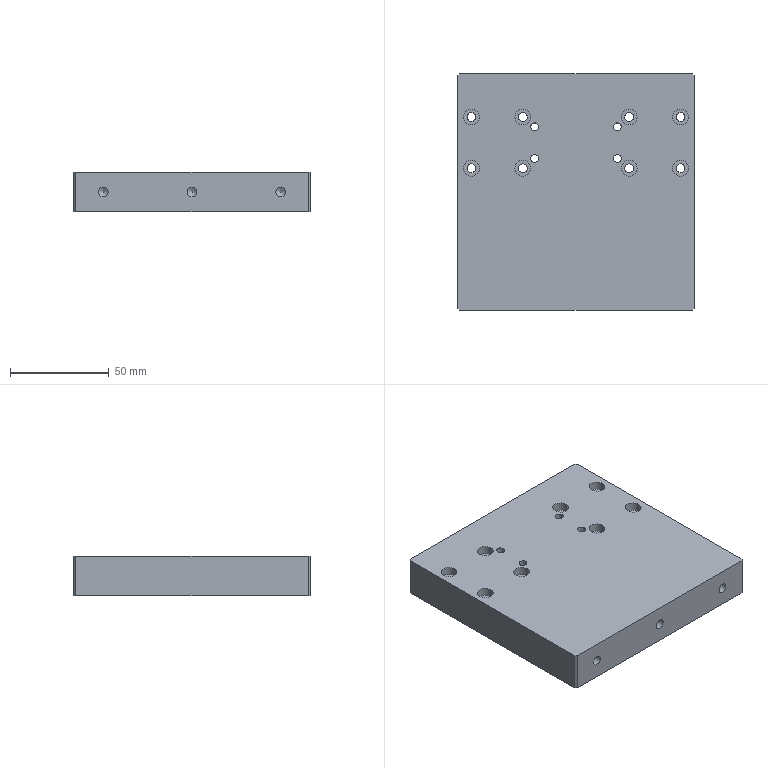Part | 1 solid | 52 faces | box 120 x 120 x 20 mm | volume 280448 mm3 | cylinder 27 | plane 18 | cone 7 | commonest cylinder face diameters 4.5 x8 8 x8 4 x4 5 x3 4.2 x2 6.8 x2
STEP:
#1=CARTESIAN_POINT('',(-59.,60.,10.));
#2=VERTEX_POINT('',#1);
#3=CARTESIAN_POINT('',(-60.,59.,10.));
#4=VERTEX_POINT('',#3);
#5=CARTESIAN_POINT('',(-59.5,59.5,10.));
#6=DIRECTION('',(-0.7071,-0.7071,0.));
#7=VECTOR('',#6,1000.);
#8=LINE('',#5,#7);
#9=EDGE_CURVE('',#2,#4,#8,.T.);
#10=ORIENTED_EDGE('',*,*,#9,.F.);
#11=CARTESIAN_POINT('',(-59.,60.,-10.));
#12=VERTEX_POINT('',#11);
#13=CARTESIAN_POINT('',(-59.,60.,10.));
#14=DIRECTION('',(0.,0.,1.));
#15=VECTOR('',#14,1000.);
#16=LINE('',#13,#15);
#17=EDGE_CURVE('',#12,#2,#16,.T.);
#18=ORIENTED_EDGE('',*,*,#17,.F.);
#19=CARTESIAN_POINT('',(-60.,59.,-10.));
#20=VERTEX_POINT('',#19);
#21=CARTESIAN_POINT('',(-60.,59.,-10.));
#22=DIRECTION('',(0.7071,0.7071,0.));
#23=VECTOR('',#22,1000.);
#24=LINE('',#21,#23);
#25=EDGE_CURVE('',#20,#12,#24,.T.);
#26=ORIENTED_EDGE('',*,*,#25,.F.);
#27=CARTESIAN_POINT('',(-60.,59.,10.));
#28=DIRECTION('',(0.,0.,-1.));
#29=VECTOR('',#28,1000.);
#30=LINE('',#27,#29);
#31=EDGE_CURVE('',#4,#20,#30,.T.);
#32=ORIENTED_EDGE('',*,*,#31,.F.);
#33=EDGE_LOOP('',(#10,#18,#26,#32));
#34=FACE_BOUND('',#33,.T.);
#35=CARTESIAN_POINT('',(-60.,59.,10.));
#36=DIRECTION('',(0.7071,-0.7071,0.));
#37=DIRECTION('',(0.,0.,-1.));
#38=AXIS2_PLACEMENT_3D('',#35,#36,#37);
#39=PLANE('',#38);
#40=ADVANCED_FACE('',(#34),#39,.F.);
#41=CARTESIAN_POINT('',(-60.,-59.,10.));
#42=VERTEX_POINT('',#41);
#43=CARTESIAN_POINT('',(-59.,-60.,10.));
#44=VERTEX_POINT('',#43);
#45=CARTESIAN_POINT('',(-59.5,-59.5,10.));
#46=DIRECTION('',(0.7071,-0.7071,0.));
#47=VECTOR('',#46,1000.);
#48=LINE('',#45,#47);
#49=EDGE_CURVE('',#42,#44,#48,.T.);
#50=ORIENTED_EDGE('',*,*,#49,.F.);
#51=CARTESIAN_POINT('',(-60.,-59.,-10.));
#52=VERTEX_POINT('',#51);
#53=CARTESIAN_POINT('',(-60.,-59.,10.));
#54=DIRECTION('',(0.,0.,1.));
#55=VECTOR('',#54,1000.);
#56=LINE('',#53,#55);
#57=EDGE_CURVE('',#52,#42,#56,.T.);
#58=ORIENTED_EDGE('',*,*,#57,.F.);
#59=CARTESIAN_POINT('',(-59.,-60.,-10.));
#60=VERTEX_POINT('',#59);
#61=CARTESIAN_POINT('',(-59.,-60.,-10.));
#62=DIRECTION('',(-0.7071,0.7071,0.));
#63=VECTOR('',#62,1000.);
#64=LINE('',#61,#63);
#65=EDGE_CURVE('',#60,#52,#64,.T.);
#66=ORIENTED_EDGE('',*,*,#65,.F.);
#67=CARTESIAN_POINT('',(-59.,-60.,10.));
#68=DIRECTION('',(0.,0.,-1.));
#69=VECTOR('',#68,1000.);
#70=LINE('',#67,#69);
#71=EDGE_CURVE('',#44,#60,#70,.T.);
#72=ORIENTED_EDGE('',*,*,#71,.F.);
#73=EDGE_LOOP('',(#50,#58,#66,#72));
#74=FACE_BOUND('',#73,.T.);
#75=CARTESIAN_POINT('',(-59.,-60.,10.));
#76=DIRECTION('',(0.7071,0.7071,0.));
#77=DIRECTION('',(0.,0.,-1.));
#78=AXIS2_PLACEMENT_3D('',#75,#76,#77);
#79=PLANE('',#78);
#80=ADVANCED_FACE('',(#74),#79,.F.);
#81=CARTESIAN_POINT('',(59.,-60.,10.));
#82=VERTEX_POINT('',#81);
#83=CARTESIAN_POINT('',(60.,-59.,10.));
#84=VERTEX_POINT('',#83);
#85=CARTESIAN_POINT('',(59.5,-59.5,10.));
#86=DIRECTION('',(0.7071,0.7071,0.));
#87=VECTOR('',#86,1000.);
#88=LINE('',#85,#87);
#89=EDGE_CURVE('',#82,#84,#88,.T.);
#90=ORIENTED_EDGE('',*,*,#89,.F.);
#91=CARTESIAN_POINT('',(59.,-60.,-10.));
#92=VERTEX_POINT('',#91);
#93=CARTESIAN_POINT('',(59.,-60.,10.));
#94=DIRECTION('',(0.,0.,1.));
#95=VECTOR('',#94,1000.);
#96=LINE('',#93,#95);
#97=EDGE_CURVE('',#92,#82,#96,.T.);
#98=ORIENTED_EDGE('',*,*,#97,.F.);
#99=CARTESIAN_POINT('',(60.,-59.,-10.));
#100=VERTEX_POINT('',#99);
#101=CARTESIAN_POINT('',(60.,-59.,-10.));
#102=DIRECTION('',(-0.7071,-0.7071,0.));
#103=VECTOR('',#102,1000.);
#104=LINE('',#101,#103);
#105=EDGE_CURVE('',#100,#92,#104,.T.);
#106=ORIENTED_EDGE('',*,*,#105,.F.);
#107=CARTESIAN_POINT('',(60.,-59.,10.));
#108=DIRECTION('',(0.,0.,-1.));
#109=VECTOR('',#108,1000.);
#110=LINE('',#107,#109);
#111=EDGE_CURVE('',#84,#100,#110,.T.);
#112=ORIENTED_EDGE('',*,*,#111,.F.);
#113=EDGE_LOOP('',(#90,#98,#106,#112));
#114=FACE_BOUND('',#113,.T.);
#115=CARTESIAN_POINT('',(60.,-59.,10.));
#116=DIRECTION('',(-0.7071,0.7071,0.));
#117=DIRECTION('',(0.,0.,-1.));
#118=AXIS2_PLACEMENT_3D('',#115,#116,#117);
#119=PLANE('',#118);
#120=ADVANCED_FACE('',(#114),#119,.F.);
#121=CARTESIAN_POINT('',(60.,59.,10.));
#122=VERTEX_POINT('',#121);
#123=CARTESIAN_POINT('',(59.,60.,10.));
#124=VERTEX_POINT('',#123);
#125=CARTESIAN_POINT('',(59.5,59.5,10.));
#126=DIRECTION('',(-0.7071,0.7071,0.));
#127=VECTOR('',#126,1000.);
#128=LINE('',#125,#127);
#129=EDGE_CURVE('',#122,#124,#128,.T.);
#130=ORIENTED_EDGE('',*,*,#129,.F.);
#131=CARTESIAN_POINT('',(60.,59.,-10.));
#132=VERTEX_POINT('',#131);
#133=CARTESIAN_POINT('',(60.,59.,10.));
#134=DIRECTION('',(0.,0.,1.));
#135=VECTOR('',#134,1000.);
#136=LINE('',#133,#135);
#137=EDGE_CURVE('',#132,#122,#136,.T.);
#138=ORIENTED_EDGE('',*,*,#137,.F.);
#139=CARTESIAN_POINT('',(59.,60.,-10.));
#140=VERTEX_POINT('',#139);
#141=CARTESIAN_POINT('',(59.,60.,-10.));
#142=DIRECTION('',(0.7071,-0.7071,0.));
#143=VECTOR('',#142,1000.);
#144=LINE('',#141,#143);
#145=EDGE_CURVE('',#140,#132,#144,.T.);
#146=ORIENTED_EDGE('',*,*,#145,.F.);
#147=CARTESIAN_POINT('',(59.,60.,10.));
#148=DIRECTION('',(0.,0.,-1.));
#149=VECTOR('',#148,1000.);
#150=LINE('',#147,#149);
#151=EDGE_CURVE('',#124,#140,#150,.T.);
#152=ORIENTED_EDGE('',*,*,#151,.F.);
#153=EDGE_LOOP('',(#130,#138,#146,#152));
#154=FACE_BOUND('',#153,.T.);
#155=CARTESIAN_POINT('',(59.,60.,10.));
#156=DIRECTION('',(-0.7071,-0.7071,0.));
#157=DIRECTION('',(0.,0.,-1.));
#158=AXIS2_PLACEMENT_3D('',#155,#156,#157);
#159=PLANE('',#158);
#160=ADVANCED_FACE('',(#154),#159,.F.);
#161=CARTESIAN_POINT('',(-49.,38.,5.6));
#162=VERTEX_POINT('',#161);
#163=CARTESIAN_POINT('',(-53.,38.,5.6));
#164=DIRECTION('',(0.,0.,1.));
#165=DIRECTION('',(1.,0.,0.));
#166=AXIS2_PLACEMENT_3D('',#163,#164,#165);
#167=CIRCLE('',#166,4.);
#168=EDGE_CURVE('',#162,#162,#167,.T.);
#169=ORIENTED_EDGE('',*,*,#168,.T.);
#170=EDGE_LOOP('',(#169));
#171=FACE_BOUND('',#170,.T.);
#172=CARTESIAN_POINT('',(-50.75,38.,5.6));
#173=VERTEX_POINT('',#172);
#174=CARTESIAN_POINT('',(-53.,38.,5.6));
#175=DIRECTION('',(0.,0.,1.));
#176=DIRECTION('',(1.,0.,0.));
#177=AXIS2_PLACEMENT_3D('',#174,#175,#176);
#178=CIRCLE('',#177,2.25);
#179=EDGE_CURVE('',#173,#173,#178,.T.);
#180=ORIENTED_EDGE('',*,*,#179,.F.);
#181=EDGE_LOOP('',(#180));
#182=FACE_BOUND('',#181,.T.);
#183=CARTESIAN_POINT('',(-50.75,38.,5.6));
#184=DIRECTION('',(0.,0.,-1.));
#185=DIRECTION('',(-1.,0.,0.));
#186=AXIS2_PLACEMENT_3D('',#183,#184,#185);
#187=PLANE('',#186);
#188=ADVANCED_FACE('',(#171,#182),#187,.F.);
#189=CARTESIAN_POINT('',(-57.,12.,5.6));
#190=VERTEX_POINT('',#189);
#191=CARTESIAN_POINT('',(-53.,12.,5.6));
#192=DIRECTION('',(0.,0.,1.));
#193=DIRECTION('',(-1.,0.,0.));
#194=AXIS2_PLACEMENT_3D('',#191,#192,#193);
#195=CIRCLE('',#194,4.);
#196=EDGE_CURVE('',#190,#190,#195,.T.);
#197=ORIENTED_EDGE('',*,*,#196,.T.);
#198=EDGE_LOOP('',(#197));
#199=FACE_BOUND('',#198,.T.);
#200=CARTESIAN_POINT('',(-55.25,12.,5.6));
#201=VERTEX_POINT('',#200);
#202=CARTESIAN_POINT('',(-53.,12.,5.6));
#203=DIRECTION('',(0.,0.,1.));
#204=DIRECTION('',(-1.,0.,0.));
#205=AXIS2_PLACEMENT_3D('',#202,#203,#204);
#206=CIRCLE('',#205,2.25);
#207=EDGE_CURVE('',#201,#201,#206,.T.);
#208=ORIENTED_EDGE('',*,*,#207,.F.);
#209=EDGE_LOOP('',(#208));
#210=FACE_BOUND('',#209,.T.);
#211=CARTESIAN_POINT('',(-50.75,38.,5.6));
#212=DIRECTION('',(0.,0.,-1.));
#213=DIRECTION('',(-1.,0.,0.));
#214=AXIS2_PLACEMENT_3D('',#211,#212,#213);
#215=PLANE('',#214);
#216=ADVANCED_FACE('',(#199,#210),#215,.F.);
#217=CARTESIAN_POINT('',(-31.,12.,5.6));
#218=VERTEX_POINT('',#217);
#219=CARTESIAN_POINT('',(-27.,12.,5.6));
#220=DIRECTION('',(0.,0.,1.));
#221=DIRECTION('',(-1.,0.,0.));
#222=AXIS2_PLACEMENT_3D('',#219,#220,#221);
#223=CIRCLE('',#222,4.);
#224=EDGE_CURVE('',#218,#218,#223,.T.);
#225=ORIENTED_EDGE('',*,*,#224,.T.);
#226=EDGE_LOOP('',(#225));
#227=FACE_BOUND('',#226,.T.);
#228=CARTESIAN_POINT('',(-29.25,12.,5.6));
#229=VERTEX_POINT('',#228);
#230=CARTESIAN_POINT('',(-27.,12.,5.6));
#231=DIRECTION('',(0.,0.,1.));
#232=DIRECTION('',(-1.,0.,0.));
#233=AXIS2_PLACEMENT_3D('',#230,#231,#232);
#234=CIRCLE('',#233,2.25);
#235=EDGE_CURVE('',#229,#229,#234,.T.);
#236=ORIENTED_EDGE('',*,*,#235,.F.);
#237=EDGE_LOOP('',(#236));
#238=FACE_BOUND('',#237,.T.);
#239=CARTESIAN_POINT('',(-50.75,38.,5.6));
#240=DIRECTION('',(0.,0.,-1.));
#241=DIRECTION('',(-1.,0.,0.));
#242=AXIS2_PLACEMENT_3D('',#239,#240,#241);
#243=PLANE('',#242);
#244=ADVANCED_FACE('',(#227,#238),#243,.F.);
#245=CARTESIAN_POINT('',(-31.,38.,5.6));
#246=VERTEX_POINT('',#245);
#247=CARTESIAN_POINT('',(-27.,38.,5.6));
#248=DIRECTION('',(0.,0.,1.));
#249=DIRECTION('',(-1.,0.,0.));
#250=AXIS2_PLACEMENT_3D('',#247,#248,#249);
#251=CIRCLE('',#250,4.);
#252=EDGE_CURVE('',#246,#246,#251,.T.);
#253=ORIENTED_EDGE('',*,*,#252,.T.);
#254=EDGE_LOOP('',(#253));
#255=FACE_BOUND('',#254,.T.);
#256=CARTESIAN_POINT('',(-29.25,38.,5.6));
#257=VERTEX_POINT('',#256);
#258=CARTESIAN_POINT('',(-27.,38.,5.6));
#259=DIRECTION('',(0.,0.,1.));
#260=DIRECTION('',(-1.,0.,0.));
#261=AXIS2_PLACEMENT_3D('',#258,#259,#260);
#262=CIRCLE('',#261,2.25);
#263=EDGE_CURVE('',#257,#257,#262,.T.);
#264=ORIENTED_EDGE('',*,*,#263,.F.);
#265=EDGE_LOOP('',(#264));
#266=FACE_BOUND('',#265,.T.);
#267=CARTESIAN_POINT('',(-50.75,38.,5.6));
#268=DIRECTION('',(0.,0.,-1.));
#269=DIRECTION('',(-1.,0.,0.));
#270=AXIS2_PLACEMENT_3D('',#267,#268,#269);
#271=PLANE('',#270);
#272=ADVANCED_FACE('',(#255,#266),#271,.F.);
#273=CARTESIAN_POINT('',(23.,38.,5.6));
#274=VERTEX_POINT('',#273);
#275=CARTESIAN_POINT('',(27.,38.,5.6));
#276=DIRECTION('',(0.,0.,1.));
#277=DIRECTION('',(-1.,0.,0.));
#278=AXIS2_PLACEMENT_3D('',#275,#276,#277);
#279=CIRCLE('',#278,4.);
#280=EDGE_CURVE('',#274,#274,#279,.T.);
#281=ORIENTED_EDGE('',*,*,#280,.T.);
#282=EDGE_LOOP('',(#281));
#283=FACE_BOUND('',#282,.T.);
#284=CARTESIAN_POINT('',(24.75,38.,5.6));
#285=VERTEX_POINT('',#284);
#286=CARTESIAN_POINT('',(27.,38.,5.6));
#287=DIRECTION('',(0.,0.,1.));
#288=DIRECTION('',(-1.,0.,0.));
#289=AXIS2_PLACEMENT_3D('',#286,#287,#288);
#290=CIRCLE('',#289,2.25);
#291=EDGE_CURVE('',#285,#285,#290,.T.);
#292=ORIENTED_EDGE('',*,*,#291,.F.);
#293=EDGE_LOOP('',(#292));
#294=FACE_BOUND('',#293,.T.);
#295=CARTESIAN_POINT('',(-50.75,38.,5.6));
#296=DIRECTION('',(0.,0.,-1.));
#297=DIRECTION('',(-1.,0.,0.));
#298=AXIS2_PLACEMENT_3D('',#295,#296,#297);
#299=PLANE('',#298);
#300=ADVANCED_FACE('',(#283,#294),#299,.F.);
#301=CARTESIAN_POINT('',(23.,12.,5.6));
#302=VERTEX_POINT('',#301);
#303=CARTESIAN_POINT('',(27.,12.,5.6));
#304=DIRECTION('',(0.,0.,1.));
#305=DIRECTION('',(-1.,0.,0.));
#306=AXIS2_PLACEMENT_3D('',#303,#304,#305);
#307=CIRCLE('',#306,4.);
#308=EDGE_CURVE('',#302,#302,#307,.T.);
#309=ORIENTED_EDGE('',*,*,#308,.T.);
#310=EDGE_LOOP('',(#309));
#311=FACE_BOUND('',#310,.T.);
#312=CARTESIAN_POINT('',(24.75,12.,5.6));
#313=VERTEX_POINT('',#312);
#314=CARTESIAN_POINT('',(27.,12.,5.6));
#315=DIRECTION('',(0.,0.,1.));
#316=DIRECTION('',(-1.,0.,0.));
#317=AXIS2_PLACEMENT_3D('',#314,#315,#316);
#318=CIRCLE('',#317,2.25);
#319=EDGE_CURVE('',#313,#313,#318,.T.);
#320=ORIENTED_EDGE('',*,*,#319,.F.);
#321=EDGE_LOOP('',(#320));
#322=FACE_BOUND('',#321,.T.);
#323=CARTESIAN_POINT('',(-50.75,38.,5.6));
#324=DIRECTION('',(0.,0.,-1.));
#325=DIRECTION('',(-1.,0.,0.));
#326=AXIS2_PLACEMENT_3D('',#323,#324,#325);
#327=PLANE('',#326);
#328=ADVANCED_FACE('',(#311,#322),#327,.F.);
#329=CARTESIAN_POINT('',(49.,12.,5.6));
#330=VERTEX_POINT('',#329);
#331=CARTESIAN_POINT('',(53.,12.,5.6));
#332=DIRECTION('',(0.,0.,1.));
#333=DIRECTION('',(-1.,0.,0.));
#334=AXIS2_PLACEMENT_3D('',#331,#332,#333);
#335=CIRCLE('',#334,4.);
#336=EDGE_CURVE('',#330,#330,#335,.T.);
#337=ORIENTED_EDGE('',*,*,#336,.T.);
#338=EDGE_LOOP('',(#337));
#339=FACE_BOUND('',#338,.T.);
#340=CARTESIAN_POINT('',(50.75,12.,5.6));
#341=VERTEX_POINT('',#340);
#342=CARTESIAN_POINT('',(53.,12.,5.6));
#343=DIRECTION('',(0.,0.,1.));
#344=DIRECTION('',(-1.,0.,0.));
#345=AXIS2_PLACEMENT_3D('',#342,#343,#344);
#346=CIRCLE('',#345,2.25);
#347=EDGE_CURVE('',#341,#341,#346,.T.);
#348=ORIENTED_EDGE('',*,*,#347,.F.);
#349=EDGE_LOOP('',(#348));
#350=FACE_BOUND('',#349,.T.);
#351=CARTESIAN_POINT('',(-50.75,38.,5.6));
#352=DIRECTION('',(0.,0.,-1.));
#353=DIRECTION('',(-1.,0.,0.));
#354=AXIS2_PLACEMENT_3D('',#351,#352,#353);
#355=PLANE('',#354);
#356=ADVANCED_FACE('',(#339,#350),#355,.F.);
#357=CARTESIAN_POINT('',(49.,38.,5.6));
#358=VERTEX_POINT('',#357);
#359=CARTESIAN_POINT('',(53.,38.,5.6));
#360=DIRECTION('',(0.,0.,1.));
#361=DIRECTION('',(-1.,0.,0.));
#362=AXIS2_PLACEMENT_3D('',#359,#360,#361);
#363=CIRCLE('',#362,4.);
#364=EDGE_CURVE('',#358,#358,#363,.T.);
#365=ORIENTED_EDGE('',*,*,#364,.T.);
#366=EDGE_LOOP('',(#365));
#367=FACE_BOUND('',#366,.T.);
#368=CARTESIAN_POINT('',(50.75,38.,5.6));
#369=VERTEX_POINT('',#368);
#370=CARTESIAN_POINT('',(53.,38.,5.6));
#371=DIRECTION('',(0.,0.,1.));
#372=DIRECTION('',(-1.,0.,0.));
#373=AXIS2_PLACEMENT_3D('',#370,#371,#372);
#374=CIRCLE('',#373,2.25);
#375=EDGE_CURVE('',#369,#369,#374,.T.);
#376=ORIENTED_EDGE('',*,*,#375,.F.);
#377=EDGE_LOOP('',(#376));
#378=FACE_BOUND('',#377,.T.);
#379=CARTESIAN_POINT('',(-50.75,38.,5.6));
#380=DIRECTION('',(0.,0.,-1.));
#381=DIRECTION('',(-1.,0.,0.));
#382=AXIS2_PLACEMENT_3D('',#379,#380,#381);
#383=PLANE('',#382);
#384=ADVANCED_FACE('',(#367,#378),#383,.F.);
#385=CARTESIAN_POINT('',(60.,60.,-10.));
#386=DIRECTION('',(-1.,0.,0.));
#387=VECTOR('',#386,1000.);
#388=LINE('',#385,#387);
#389=EDGE_CURVE('',#140,#12,#388,.T.);
#390=ORIENTED_EDGE('',*,*,#389,.F.);
#391=ORIENTED_EDGE('',*,*,#145,.T.);
#392=CARTESIAN_POINT('',(60.,-60.,-10.));
#393=DIRECTION('',(0.,1.,0.));
#394=VECTOR('',#393,1000.);
#395=LINE('',#392,#394);
#396=EDGE_CURVE('',#100,#132,#395,.T.);
#397=ORIENTED_EDGE('',*,*,#396,.F.);
#398=ORIENTED_EDGE('',*,*,#105,.T.);
#399=CARTESIAN_POINT('',(60.,-60.,-10.));
#400=DIRECTION('',(1.,0.,0.));
#401=VECTOR('',#400,1000.);
#402=LINE('',#399,#401);
#403=EDGE_CURVE('',#60,#92,#402,.T.);
#404=ORIENTED_EDGE('',*,*,#403,.F.);
#405=ORIENTED_EDGE('',*,*,#65,.T.);
#406=CARTESIAN_POINT('',(-60.,-60.,-10.));
#407=DIRECTION('',(0.,-1.,0.));
#408=VECTOR('',#407,1000.);
#409=LINE('',#406,#408);
#410=EDGE_CURVE('',#20,#52,#409,.T.);
#411=ORIENTED_EDGE('',*,*,#410,.F.);
#412=ORIENTED_EDGE('',*,*,#25,.T.);
#413=EDGE_LOOP('',(#390,#391,#397,#398,#404,#405,#411,#412));
#414=FACE_BOUND('',#413,.T.);
#415=CARTESIAN_POINT('',(55.25,38.,-10.));
#416=VERTEX_POINT('',#415);
#417=CARTESIAN_POINT('',(53.,38.,-10.));
#418=DIRECTION('',(0.,0.,1.));
#419=DIRECTION('',(1.,0.,0.));
#420=AXIS2_PLACEMENT_3D('',#417,#418,#419);
#421=CIRCLE('',#420,2.25);
#422=EDGE_CURVE('',#416,#416,#421,.T.);
#423=ORIENTED_EDGE('',*,*,#422,.T.);
#424=EDGE_LOOP('',(#423));
#425=FACE_BOUND('',#424,.T.);
#426=CARTESIAN_POINT('',(55.25,12.,-10.));
#427=VERTEX_POINT('',#426);
#428=CARTESIAN_POINT('',(53.,12.,-10.));
#429=DIRECTION('',(0.,0.,1.));
#430=DIRECTION('',(1.,0.,0.));
#431=AXIS2_PLACEMENT_3D('',#428,#429,#430);
#432=CIRCLE('',#431,2.25);
#433=EDGE_CURVE('',#427,#427,#432,.T.);
#434=ORIENTED_EDGE('',*,*,#433,.T.);
#435=EDGE_LOOP('',(#434));
#436=FACE_BOUND('',#435,.T.);
#437=CARTESIAN_POINT('',(29.25,12.,-10.));
#438=VERTEX_POINT('',#437);
#439=CARTESIAN_POINT('',(27.,12.,-10.));
#440=DIRECTION('',(0.,0.,1.));
#441=DIRECTION('',(1.,0.,0.));
#442=AXIS2_PLACEMENT_3D('',#439,#440,#441);
#443=CIRCLE('',#442,2.25);
#444=EDGE_CURVE('',#438,#438,#443,.T.);
#445=ORIENTED_EDGE('',*,*,#444,.T.);
#446=EDGE_LOOP('',(#445));
#447=FACE_BOUND('',#446,.T.);
#448=CARTESIAN_POINT('',(29.25,38.,-10.));
#449=VERTEX_POINT('',#448);
#450=CARTESIAN_POINT('',(27.,38.,-10.));
#451=DIRECTION('',(0.,0.,1.));
#452=DIRECTION('',(1.,0.,0.));
#453=AXIS2_PLACEMENT_3D('',#450,#451,#452);
#454=CIRCLE('',#453,2.25);
#455=EDGE_CURVE('',#449,#449,#454,.T.);
#456=ORIENTED_EDGE('',*,*,#455,.T.);
#457=EDGE_LOOP('',(#456));
#458=FACE_BOUND('',#457,.T.);
#459=CARTESIAN_POINT('',(-24.75,38.,-10.));
#460=VERTEX_POINT('',#459);
#461=CARTESIAN_POINT('',(-27.,38.,-10.));
#462=DIRECTION('',(0.,0.,1.));
#463=DIRECTION('',(1.,0.,0.));
#464=AXIS2_PLACEMENT_3D('',#461,#462,#463);
#465=CIRCLE('',#464,2.25);
#466=EDGE_CURVE('',#460,#460,#465,.T.);
#467=ORIENTED_EDGE('',*,*,#466,.T.);
#468=EDGE_LOOP('',(#467));
#469=FACE_BOUND('',#468,.T.);
#470=CARTESIAN_POINT('',(-24.75,12.,-10.));
#471=VERTEX_POINT('',#470);
#472=CARTESIAN_POINT('',(-27.,12.,-10.));
#473=DIRECTION('',(0.,0.,1.));
#474=DIRECTION('',(1.,0.,0.));
#475=AXIS2_PLACEMENT_3D('',#472,#473,#474);
#476=CIRCLE('',#475,2.25);
#477=EDGE_CURVE('',#471,#471,#476,.T.);
#478=ORIENTED_EDGE('',*,*,#477,.T.);
#479=EDGE_LOOP('',(#478));
#480=FACE_BOUND('',#479,.T.);
#481=CARTESIAN_POINT('',(-50.75,12.,-10.));
#482=VERTEX_POINT('',#481);
#483=CARTESIAN_POINT('',(-53.,12.,-10.));
#484=DIRECTION('',(0.,0.,1.));
#485=DIRECTION('',(1.,0.,0.));
#486=AXIS2_PLACEMENT_3D('',#483,#484,#485);
#487=CIRCLE('',#486,2.25);
#488=EDGE_CURVE('',#482,#482,#487,.T.);
#489=ORIENTED_EDGE('',*,*,#488,.T.);
#490=EDGE_LOOP('',(#489));
#491=FACE_BOUND('',#490,.T.);
#492=CARTESIAN_POINT('',(-50.75,38.,-10.));
#493=VERTEX_POINT('',#492);
#494=CARTESIAN_POINT('',(-53.,38.,-10.));
#495=DIRECTION('',(0.,0.,1.));
#496=DIRECTION('',(1.,0.,0.));
#497=AXIS2_PLACEMENT_3D('',#494,#495,#496);
#498=CIRCLE('',#497,2.25);
#499=EDGE_CURVE('',#493,#493,#498,.T.);
#500=ORIENTED_EDGE('',*,*,#499,.T.);
#501=EDGE_LOOP('',(#500));
#502=FACE_BOUND('',#501,.T.);
#503=CARTESIAN_POINT('',(23.,17.,-10.));
#504=VERTEX_POINT('',#503);
#505=CARTESIAN_POINT('',(21.,17.,-10.));
#506=DIRECTION('',(0.,0.,1.));
#507=DIRECTION('',(1.,0.,0.));
#508=AXIS2_PLACEMENT_3D('',#505,#506,#507);
#509=CIRCLE('',#508,2.);
#510=EDGE_CURVE('',#504,#504,#509,.T.);
#511=ORIENTED_EDGE('',*,*,#510,.T.);
#512=EDGE_LOOP('',(#511));
#513=FACE_BOUND('',#512,.T.);
#514=CARTESIAN_POINT('',(23.,33.,-10.));
#515=VERTEX_POINT('',#514);
#516=CARTESIAN_POINT('',(21.,33.,-10.));
#517=DIRECTION('',(0.,0.,1.));
#518=DIRECTION('',(1.,0.,0.));
#519=AXIS2_PLACEMENT_3D('',#516,#517,#518);
#520=CIRCLE('',#519,2.);
#521=EDGE_CURVE('',#515,#515,#520,.T.);
#522=ORIENTED_EDGE('',*,*,#521,.T.);
#523=EDGE_LOOP('',(#522));
#524=FACE_BOUND('',#523,.T.);
#525=CARTESIAN_POINT('',(-19.,17.,-10.));
#526=VERTEX_POINT('',#525);
#527=CARTESIAN_POINT('',(-21.,17.,-10.));
#528=DIRECTION('',(0.,0.,1.));
#529=DIRECTION('',(1.,0.,0.));
#530=AXIS2_PLACEMENT_3D('',#527,#528,#529);
#531=CIRCLE('',#530,2.);
#532=EDGE_CURVE('',#526,#526,#531,.T.);
#533=ORIENTED_EDGE('',*,*,#532,.T.);
#534=EDGE_LOOP('',(#533));
#535=FACE_BOUND('',#534,.T.);
#536=CARTESIAN_POINT('',(-19.,33.,-10.));
#537=VERTEX_POINT('',#536);
#538=CARTESIAN_POINT('',(-21.,33.,-10.));
#539=DIRECTION('',(0.,0.,1.));
#540=DIRECTION('',(1.,0.,0.));
#541=AXIS2_PLACEMENT_3D('',#538,#539,#540);
#542=CIRCLE('',#541,2.);
#543=EDGE_CURVE('',#537,#537,#542,.T.);
#544=ORIENTED_EDGE('',*,*,#543,.T.);
#545=EDGE_LOOP('',(#544));
#546=FACE_BOUND('',#545,.T.);
#547=CARTESIAN_POINT('',(0.,0.,-10.));
#548=DIRECTION('',(0.,0.,1.));
#549=DIRECTION('',(1.,0.,0.));
#550=AXIS2_PLACEMENT_3D('',#547,#548,#549);
#551=PLANE('',#550);
#552=ADVANCED_FACE('',(#414,#425,#436,#447,#458,#469,#480,#491,#502,#513,#524,#535,#546),#551,.F.);
#553=CARTESIAN_POINT('',(60.,-60.,10.));
#554=DIRECTION('',(0.,1.,0.));
#555=VECTOR('',#554,1000.);
#556=LINE('',#553,#555);
#557=EDGE_CURVE('',#84,#122,#556,.T.);
#558=ORIENTED_EDGE('',*,*,#557,.T.);
#559=ORIENTED_EDGE('',*,*,#129,.T.);
#560=CARTESIAN_POINT('',(60.,60.,10.));
#561=DIRECTION('',(-1.,0.,0.));
#562=VECTOR('',#561,1000.);
#563=LINE('',#560,#562);
#564=EDGE_CURVE('',#124,#2,#563,.T.);
#565=ORIENTED_EDGE('',*,*,#564,.T.);
#566=ORIENTED_EDGE('',*,*,#9,.T.);
#567=CARTESIAN_POINT('',(-60.,-60.,10.));
#568=DIRECTION('',(0.,-1.,0.));
#569=VECTOR('',#568,1000.);
#570=LINE('',#567,#569);
#571=EDGE_CURVE('',#4,#42,#570,.T.);
#572=ORIENTED_EDGE('',*,*,#571,.T.);
#573=ORIENTED_EDGE('',*,*,#49,.T.);
#574=CARTESIAN_POINT('',(60.,-60.,10.));
#575=DIRECTION('',(1.,0.,0.));
#576=VECTOR('',#575,1000.);
#577=LINE('',#574,#576);
#578=EDGE_CURVE('',#44,#82,#577,.T.);
#579=ORIENTED_EDGE('',*,*,#578,.T.);
#580=ORIENTED_EDGE('',*,*,#89,.T.);
#581=EDGE_LOOP('',(#558,#559,#565,#566,#572,#573,#579,#580));
#582=FACE_BOUND('',#581,.T.);
#583=CARTESIAN_POINT('',(57.,38.,10.));
#584=VERTEX_POINT('',#583);
#585=CARTESIAN_POINT('',(53.,38.,10.));
#586=DIRECTION('',(0.,0.,1.));
#587=DIRECTION('',(1.,0.,0.));
#588=AXIS2_PLACEMENT_3D('',#585,#586,#587);
#589=CIRCLE('',#588,4.);
#590=EDGE_CURVE('',#584,#584,#589,.T.);
#591=ORIENTED_EDGE('',*,*,#590,.F.);
#592=EDGE_LOOP('',(#591));
#593=FACE_BOUND('',#592,.T.);
#594=CARTESIAN_POINT('',(57.,12.,10.));
#595=VERTEX_POINT('',#594);
#596=CARTESIAN_POINT('',(53.,12.,10.));
#597=DIRECTION('',(0.,0.,1.));
#598=DIRECTION('',(1.,0.,0.));
#599=AXIS2_PLACEMENT_3D('',#596,#597,#598);
#600=CIRCLE('',#599,4.);
#601=EDGE_CURVE('',#595,#595,#600,.T.);
#602=ORIENTED_EDGE('',*,*,#601,.F.);
#603=EDGE_LOOP('',(#602));
#604=FACE_BOUND('',#603,.T.);
#605=CARTESIAN_POINT('',(31.,12.,10.));
#606=VERTEX_POINT('',#605);
#607=CARTESIAN_POINT('',(27.,12.,10.));
#608=DIRECTION('',(0.,0.,1.));
#609=DIRECTION('',(1.,0.,0.));
#610=AXIS2_PLACEMENT_3D('',#607,#608,#609);
#611=CIRCLE('',#610,4.);
#612=EDGE_CURVE('',#606,#606,#611,.T.);
#613=ORIENTED_EDGE('',*,*,#612,.F.);
#614=EDGE_LOOP('',(#613));
#615=FACE_BOUND('',#614,.T.);
#616=CARTESIAN_POINT('',(31.,38.,10.));
#617=VERTEX_POINT('',#616);
#618=CARTESIAN_POINT('',(27.,38.,10.));
#619=DIRECTION('',(0.,0.,1.));
#620=DIRECTION('',(1.,0.,0.));
#621=AXIS2_PLACEMENT_3D('',#618,#619,#620);
#622=CIRCLE('',#621,4.);
#623=EDGE_CURVE('',#617,#617,#622,.T.);
#624=ORIENTED_EDGE('',*,*,#623,.F.);
#625=EDGE_LOOP('',(#624));
#626=FACE_BOUND('',#625,.T.);
#627=CARTESIAN_POINT('',(-23.,38.,10.));
#628=VERTEX_POINT('',#627);
#629=CARTESIAN_POINT('',(-27.,38.,10.));
#630=DIRECTION('',(0.,0.,1.));
#631=DIRECTION('',(1.,0.,0.));
#632=AXIS2_PLACEMENT_3D('',#629,#630,#631);
#633=CIRCLE('',#632,4.);
#634=EDGE_CURVE('',#628,#628,#633,.T.);
#635=ORIENTED_EDGE('',*,*,#634,.F.);
#636=EDGE_LOOP('',(#635));
#637=FACE_BOUND('',#636,.T.);
#638=CARTESIAN_POINT('',(-23.,12.,10.));
#639=VERTEX_POINT('',#638);
#640=CARTESIAN_POINT('',(-27.,12.,10.));
#641=DIRECTION('',(0.,0.,1.));
#642=DIRECTION('',(1.,0.,0.));
#643=AXIS2_PLACEMENT_3D('',#640,#641,#642);
#644=CIRCLE('',#643,4.);
#645=EDGE_CURVE('',#639,#639,#644,.T.);
#646=ORIENTED_EDGE('',*,*,#645,.F.);
#647=EDGE_LOOP('',(#646));
#648=FACE_BOUND('',#647,.T.);
#649=CARTESIAN_POINT('',(-49.,12.,10.));
#650=VERTEX_POINT('',#649);
#651=CARTESIAN_POINT('',(-53.,12.,10.));
#652=DIRECTION('',(0.,0.,1.));
#653=DIRECTION('',(1.,0.,0.));
#654=AXIS2_PLACEMENT_3D('',#651,#652,#653);
#655=CIRCLE('',#654,4.);
#656=EDGE_CURVE('',#650,#650,#655,.T.);
#657=ORIENTED_EDGE('',*,*,#656,.F.);
#658=EDGE_LOOP('',(#657));
#659=FACE_BOUND('',#658,.T.);
#660=CARTESIAN_POINT('',(-49.,38.,10.));
#661=VERTEX_POINT('',#660);
#662=CARTESIAN_POINT('',(-53.,38.,10.));
#663=DIRECTION('',(0.,0.,1.));
#664=DIRECTION('',(1.,0.,0.));
#665=AXIS2_PLACEMENT_3D('',#662,#663,#664);
#666=CIRCLE('',#665,4.);
#667=EDGE_CURVE('',#661,#661,#666,.T.);
#668=ORIENTED_EDGE('',*,*,#667,.F.);
#669=EDGE_LOOP('',(#668));
#670=FACE_BOUND('',#669,.T.);
#671=CARTESIAN_POINT('',(23.,17.,10.));
#672=VERTEX_POINT('',#671);
#673=CARTESIAN_POINT('',(21.,17.,10.));
#674=DIRECTION('',(0.,0.,1.));
#675=DIRECTION('',(1.,0.,0.));
#676=AXIS2_PLACEMENT_3D('',#673,#674,#675);
#677=CIRCLE('',#676,2.);
#678=EDGE_CURVE('',#672,#672,#677,.T.);
#679=ORIENTED_EDGE('',*,*,#678,.F.);
#680=EDGE_LOOP('',(#679));
#681=FACE_BOUND('',#680,.T.);
#682=CARTESIAN_POINT('',(23.,33.,10.));
#683=VERTEX_POINT('',#682);
#684=CARTESIAN_POINT('',(21.,33.,10.));
#685=DIRECTION('',(0.,0.,1.));
#686=DIRECTION('',(1.,0.,0.));
#687=AXIS2_PLACEMENT_3D('',#684,#685,#686);
#688=CIRCLE('',#687,2.);
#689=EDGE_CURVE('',#683,#683,#688,.T.);
#690=ORIENTED_EDGE('',*,*,#689,.F.);
#691=EDGE_LOOP('',(#690));
#692=FACE_BOUND('',#691,.T.);
#693=CARTESIAN_POINT('',(-19.,17.,10.));
#694=VERTEX_POINT('',#693);
#695=CARTESIAN_POINT('',(-21.,17.,10.));
#696=DIRECTION('',(0.,0.,1.));
#697=DIRECTION('',(1.,0.,0.));
#698=AXIS2_PLACEMENT_3D('',#695,#696,#697);
#699=CIRCLE('',#698,2.);
#700=EDGE_CURVE('',#694,#694,#699,.T.);
#701=ORIENTED_EDGE('',*,*,#700,.F.);
#702=EDGE_LOOP('',(#701));
#703=FACE_BOUND('',#702,.T.);
#704=CARTESIAN_POINT('',(-19.,33.,10.));
#705=VERTEX_POINT('',#704);
#706=CARTESIAN_POINT('',(-21.,33.,10.));
#707=DIRECTION('',(0.,0.,1.));
#708=DIRECTION('',(1.,0.,0.));
#709=AXIS2_PLACEMENT_3D('',#706,#707,#708);
#710=CIRCLE('',#709,2.);
#711=EDGE_CURVE('',#705,#705,#710,.T.);
#712=ORIENTED_EDGE('',*,*,#711,.F.);
#713=EDGE_LOOP('',(#712));
#714=FACE_BOUND('',#713,.T.);
#715=CARTESIAN_POINT('',(0.,0.,10.));
#716=DIRECTION('',(0.,0.,1.));
#717=DIRECTION('',(1.,0.,0.));
#718=AXIS2_PLACEMENT_3D('',#715,#716,#717);
#719=PLANE('',#718);
#720=ADVANCED_FACE('',(#582,#593,#604,#615,#626,#637,#648,#659,#670,#681,#692,#703,#714),#719,.T.);
#721=ORIENTED_EDGE('',*,*,#564,.F.);
#722=ORIENTED_EDGE('',*,*,#151,.T.);
#723=ORIENTED_EDGE('',*,*,#389,.T.);
#724=ORIENTED_EDGE('',*,*,#17,.T.);
#725=EDGE_LOOP('',(#721,#722,#723,#724));
#726=FACE_BOUND('',#725,.T.);
#727=CARTESIAN_POINT('',(40.,60.,3.4));
#728=VERTEX_POINT('',#727);
#729=CARTESIAN_POINT('',(40.,60.,0.));
#730=DIRECTION('',(0.,1.,0.));
#731=DIRECTION('',(0.,0.,1.));
#732=AXIS2_PLACEMENT_3D('',#729,#730,#731);
#733=CIRCLE('',#732,3.4);
#734=EDGE_CURVE('',#728,#728,#733,.T.);
#735=ORIENTED_EDGE('',*,*,#734,.F.);
#736=EDGE_LOOP('',(#735));
#737=FACE_BOUND('',#736,.T.);
#738=CARTESIAN_POINT('',(-40.,60.,3.4));
#739=VERTEX_POINT('',#738);
#740=CARTESIAN_POINT('',(-40.,60.,0.));
#741=DIRECTION('',(0.,1.,0.));
#742=DIRECTION('',(0.,0.,1.));
#743=AXIS2_PLACEMENT_3D('',#740,#741,#742);
#744=CIRCLE('',#743,3.4);
#745=EDGE_CURVE('',#739,#739,#744,.T.);
#746=ORIENTED_EDGE('',*,*,#745,.F.);
#747=EDGE_LOOP('',(#746));
#748=FACE_BOUND('',#747,.T.);
#749=CARTESIAN_POINT('',(10.,60.,2.1));
#750=VERTEX_POINT('',#749);
#751=CARTESIAN_POINT('',(10.,60.,0.));
#752=DIRECTION('',(0.,1.,0.));
#753=DIRECTION('',(0.,0.,1.));
#754=AXIS2_PLACEMENT_3D('',#751,#752,#753);
#755=CIRCLE('',#754,2.1);
#756=EDGE_CURVE('',#750,#750,#755,.T.);
#757=ORIENTED_EDGE('',*,*,#756,.F.);
#758=EDGE_LOOP('',(#757));
#759=FACE_BOUND('',#758,.T.);
#760=CARTESIAN_POINT('',(-10.,60.,2.1));
#761=VERTEX_POINT('',#760);
#762=CARTESIAN_POINT('',(-10.,60.,0.));
#763=DIRECTION('',(0.,1.,0.));
#764=DIRECTION('',(0.,0.,1.));
#765=AXIS2_PLACEMENT_3D('',#762,#763,#764);
#766=CIRCLE('',#765,2.1);
#767=EDGE_CURVE('',#761,#761,#766,.T.);
#768=ORIENTED_EDGE('',*,*,#767,.F.);
#769=EDGE_LOOP('',(#768));
#770=FACE_BOUND('',#769,.T.);
#771=CARTESIAN_POINT('',(60.,60.,10.));
#772=DIRECTION('',(0.,-1.,0.));
#773=DIRECTION('',(1.,0.,0.));
#774=AXIS2_PLACEMENT_3D('',#771,#772,#773);
#775=PLANE('',#774);
#776=ADVANCED_FACE('',(#726,#737,#748,#759,#770),#775,.F.);
#777=ORIENTED_EDGE('',*,*,#396,.T.);
#778=ORIENTED_EDGE('',*,*,#137,.T.);
#779=ORIENTED_EDGE('',*,*,#557,.F.);
#780=ORIENTED_EDGE('',*,*,#111,.T.);
#781=EDGE_LOOP('',(#777,#778,#779,#780));
#782=FACE_BOUND('',#781,.T.);
#783=CARTESIAN_POINT('',(60.,-60.,10.));
#784=DIRECTION('',(-1.,0.,0.));
#785=DIRECTION('',(0.,0.,1.));
#786=AXIS2_PLACEMENT_3D('',#783,#784,#785);
#787=PLANE('',#786);
#788=ADVANCED_FACE('',(#782),#787,.F.);
#789=ORIENTED_EDGE('',*,*,#403,.T.);
#790=ORIENTED_EDGE('',*,*,#97,.T.);
#791=ORIENTED_EDGE('',*,*,#578,.F.);
#792=ORIENTED_EDGE('',*,*,#71,.T.);
#793=EDGE_LOOP('',(#789,#790,#791,#792));
#794=FACE_BOUND('',#793,.T.);
#795=CARTESIAN_POINT('',(-45.,-60.,-2.5));
#796=VERTEX_POINT('',#795);
#797=CARTESIAN_POINT('',(-45.,-60.,0.));
#798=DIRECTION('',(0.,-1.,0.));
#799=DIRECTION('',(0.,0.,-1.));
#800=AXIS2_PLACEMENT_3D('',#797,#798,#799);
#801=CIRCLE('',#800,2.5);
#802=EDGE_CURVE('',#796,#796,#801,.T.);
#803=ORIENTED_EDGE('',*,*,#802,.F.);
#804=EDGE_LOOP('',(#803));
#805=FACE_BOUND('',#804,.T.);
#806=CARTESIAN_POINT('',(0.,-60.,-2.5));
#807=VERTEX_POINT('',#806);
#808=CARTESIAN_POINT('',(0.,-60.,0.));
#809=DIRECTION('',(0.,-1.,0.));
#810=DIRECTION('',(0.,0.,-1.));
#811=AXIS2_PLACEMENT_3D('',#808,#809,#810);
#812=CIRCLE('',#811,2.5);
#813=EDGE_CURVE('',#807,#807,#812,.T.);
#814=ORIENTED_EDGE('',*,*,#813,.F.);
#815=EDGE_LOOP('',(#814));
#816=FACE_BOUND('',#815,.T.);
#817=CARTESIAN_POINT('',(45.,-60.,-2.5));
#818=VERTEX_POINT('',#817);
#819=CARTESIAN_POINT('',(45.,-60.,0.));
#820=DIRECTION('',(0.,-1.,0.));
#821=DIRECTION('',(0.,0.,-1.));
#822=AXIS2_PLACEMENT_3D('',#819,#820,#821);
#823=CIRCLE('',#822,2.5);
#824=EDGE_CURVE('',#818,#818,#823,.T.);
#825=ORIENTED_EDGE('',*,*,#824,.F.);
#826=EDGE_LOOP('',(#825));
#827=FACE_BOUND('',#826,.T.);
#828=CARTESIAN_POINT('',(60.,-60.,10.));
#829=DIRECTION('',(0.,1.,0.));
#830=DIRECTION('',(-1.,0.,0.));
#831=AXIS2_PLACEMENT_3D('',#828,#829,#830);
#832=PLANE('',#831);
#833=ADVANCED_FACE('',(#794,#805,#816,#827),#832,.F.);
#834=ORIENTED_EDGE('',*,*,#410,.T.);
#835=ORIENTED_EDGE('',*,*,#57,.T.);
#836=ORIENTED_EDGE('',*,*,#571,.F.);
#837=ORIENTED_EDGE('',*,*,#31,.T.);
#838=EDGE_LOOP('',(#834,#835,#836,#837));
#839=FACE_BOUND('',#838,.T.);
#840=CARTESIAN_POINT('',(-60.,-60.,10.));
#841=DIRECTION('',(1.,0.,0.));
#842=DIRECTION('',(0.,0.,-1.));
#843=AXIS2_PLACEMENT_3D('',#840,#841,#842);
#844=PLANE('',#843);
#845=ADVANCED_FACE('',(#839),#844,.F.);
#846=ORIENTED_EDGE('',*,*,#422,.F.);
#847=EDGE_LOOP('',(#846));
#848=FACE_BOUND('',#847,.T.);
#849=ORIENTED_EDGE('',*,*,#375,.T.);
#850=EDGE_LOOP('',(#849));
#851=FACE_BOUND('',#850,.T.);
#852=CARTESIAN_POINT('',(53.,38.,10.));
#853=DIRECTION('',(0.,0.,1.));
#854=DIRECTION('',(1.,0.,0.));
#855=AXIS2_PLACEMENT_3D('',#852,#853,#854);
#856=CYLINDRICAL_SURFACE('',#855,2.25);
#857=ADVANCED_FACE('',(#848,#851),#856,.F.);
#858=ORIENTED_EDGE('',*,*,#364,.F.);
#859=EDGE_LOOP('',(#858));
#860=FACE_BOUND('',#859,.T.);
#861=ORIENTED_EDGE('',*,*,#590,.T.);
#862=EDGE_LOOP('',(#861));
#863=FACE_BOUND('',#862,.T.);
#864=CARTESIAN_POINT('',(53.,38.,10.));
#865=DIRECTION('',(0.,0.,1.));
#866=DIRECTION('',(1.,0.,0.));
#867=AXIS2_PLACEMENT_3D('',#864,#865,#866);
#868=CYLINDRICAL_SURFACE('',#867,4.);
#869=ADVANCED_FACE('',(#860,#863),#868,.F.);
#870=ORIENTED_EDGE('',*,*,#433,.F.);
#871=EDGE_LOOP('',(#870));
#872=FACE_BOUND('',#871,.T.);
#873=ORIENTED_EDGE('',*,*,#347,.T.);
#874=EDGE_LOOP('',(#873));
#875=FACE_BOUND('',#874,.T.);
#876=CARTESIAN_POINT('',(53.,12.,10.));
#877=DIRECTION('',(0.,0.,1.));
#878=DIRECTION('',(1.,0.,0.));
#879=AXIS2_PLACEMENT_3D('',#876,#877,#878);
#880=CYLINDRICAL_SURFACE('',#879,2.25);
#881=ADVANCED_FACE('',(#872,#875),#880,.F.);
#882=ORIENTED_EDGE('',*,*,#336,.F.);
#883=EDGE_LOOP('',(#882));
#884=FACE_BOUND('',#883,.T.);
#885=ORIENTED_EDGE('',*,*,#601,.T.);
#886=EDGE_LOOP('',(#885));
#887=FACE_BOUND('',#886,.T.);
#888=CARTESIAN_POINT('',(53.,12.,10.));
#889=DIRECTION('',(0.,0.,1.));
#890=DIRECTION('',(1.,0.,0.));
#891=AXIS2_PLACEMENT_3D('',#888,#889,#890);
#892=CYLINDRICAL_SURFACE('',#891,4.);
#893=ADVANCED_FACE('',(#884,#887),#892,.F.);
#894=ORIENTED_EDGE('',*,*,#444,.F.);
#895=EDGE_LOOP('',(#894));
#896=FACE_BOUND('',#895,.T.);
#897=ORIENTED_EDGE('',*,*,#319,.T.);
#898=EDGE_LOOP('',(#897));
#899=FACE_BOUND('',#898,.T.);
#900=CARTESIAN_POINT('',(27.,12.,10.));
#901=DIRECTION('',(0.,0.,1.));
#902=DIRECTION('',(1.,0.,0.));
#903=AXIS2_PLACEMENT_3D('',#900,#901,#902);
#904=CYLINDRICAL_SURFACE('',#903,2.25);
#905=ADVANCED_FACE('',(#896,#899),#904,.F.);
#906=ORIENTED_EDGE('',*,*,#308,.F.);
#907=EDGE_LOOP('',(#906));
#908=FACE_BOUND('',#907,.T.);
#909=ORIENTED_EDGE('',*,*,#612,.T.);
#910=EDGE_LOOP('',(#909));
#911=FACE_BOUND('',#910,.T.);
#912=CARTESIAN_POINT('',(27.,12.,10.));
#913=DIRECTION('',(0.,0.,1.));
#914=DIRECTION('',(1.,0.,0.));
#915=AXIS2_PLACEMENT_3D('',#912,#913,#914);
#916=CYLINDRICAL_SURFACE('',#915,4.);
#917=ADVANCED_FACE('',(#908,#911),#916,.F.);
#918=ORIENTED_EDGE('',*,*,#455,.F.);
#919=EDGE_LOOP('',(#918));
#920=FACE_BOUND('',#919,.T.);
#921=ORIENTED_EDGE('',*,*,#291,.T.);
#922=EDGE_LOOP('',(#921));
#923=FACE_BOUND('',#922,.T.);
#924=CARTESIAN_POINT('',(27.,38.,10.));
#925=DIRECTION('',(0.,0.,1.));
#926=DIRECTION('',(1.,0.,0.));
#927=AXIS2_PLACEMENT_3D('',#924,#925,#926);
#928=CYLINDRICAL_SURFACE('',#927,2.25);
#929=ADVANCED_FACE('',(#920,#923),#928,.F.);
#930=ORIENTED_EDGE('',*,*,#280,.F.);
#931=EDGE_LOOP('',(#930));
#932=FACE_BOUND('',#931,.T.);
#933=ORIENTED_EDGE('',*,*,#623,.T.);
#934=EDGE_LOOP('',(#933));
#935=FACE_BOUND('',#934,.T.);
#936=CARTESIAN_POINT('',(27.,38.,10.));
#937=DIRECTION('',(0.,0.,1.));
#938=DIRECTION('',(1.,0.,0.));
#939=AXIS2_PLACEMENT_3D('',#936,#937,#938);
#940=CYLINDRICAL_SURFACE('',#939,4.);
#941=ADVANCED_FACE('',(#932,#935),#940,.F.);
#942=ORIENTED_EDGE('',*,*,#466,.F.);
#943=EDGE_LOOP('',(#942));
#944=FACE_BOUND('',#943,.T.);
#945=ORIENTED_EDGE('',*,*,#263,.T.);
#946=EDGE_LOOP('',(#945));
#947=FACE_BOUND('',#946,.T.);
#948=CARTESIAN_POINT('',(-27.,38.,10.));
#949=DIRECTION('',(0.,0.,1.));
#950=DIRECTION('',(1.,0.,0.));
#951=AXIS2_PLACEMENT_3D('',#948,#949,#950);
#952=CYLINDRICAL_SURFACE('',#951,2.25);
#953=ADVANCED_FACE('',(#944,#947),#952,.F.);
#954=ORIENTED_EDGE('',*,*,#252,.F.);
#955=EDGE_LOOP('',(#954));
#956=FACE_BOUND('',#955,.T.);
#957=ORIENTED_EDGE('',*,*,#634,.T.);
#958=EDGE_LOOP('',(#957));
#959=FACE_BOUND('',#958,.T.);
#960=CARTESIAN_POINT('',(-27.,38.,10.));
#961=DIRECTION('',(0.,0.,1.));
#962=DIRECTION('',(1.,0.,0.));
#963=AXIS2_PLACEMENT_3D('',#960,#961,#962);
#964=CYLINDRICAL_SURFACE('',#963,4.);
#965=ADVANCED_FACE('',(#956,#959),#964,.F.);
#966=ORIENTED_EDGE('',*,*,#477,.F.);
#967=EDGE_LOOP('',(#966));
#968=FACE_BOUND('',#967,.T.);
#969=ORIENTED_EDGE('',*,*,#235,.T.);
#970=EDGE_LOOP('',(#969));
#971=FACE_BOUND('',#970,.T.);
#972=CARTESIAN_POINT('',(-27.,12.,10.));
#973=DIRECTION('',(0.,0.,1.));
#974=DIRECTION('',(1.,0.,0.));
#975=AXIS2_PLACEMENT_3D('',#972,#973,#974);
#976=CYLINDRICAL_SURFACE('',#975,2.25);
#977=ADVANCED_FACE('',(#968,#971),#976,.F.);
#978=ORIENTED_EDGE('',*,*,#224,.F.);
#979=EDGE_LOOP('',(#978));
#980=FACE_BOUND('',#979,.T.);
#981=ORIENTED_EDGE('',*,*,#645,.T.);
#982=EDGE_LOOP('',(#981));
#983=FACE_BOUND('',#982,.T.);
#984=CARTESIAN_POINT('',(-27.,12.,10.));
#985=DIRECTION('',(0.,0.,1.));
#986=DIRECTION('',(1.,0.,0.));
#987=AXIS2_PLACEMENT_3D('',#984,#985,#986);
#988=CYLINDRICAL_SURFACE('',#987,4.);
#989=ADVANCED_FACE('',(#980,#983),#988,.F.);
#990=ORIENTED_EDGE('',*,*,#488,.F.);
#991=EDGE_LOOP('',(#990));
#992=FACE_BOUND('',#991,.T.);
#993=ORIENTED_EDGE('',*,*,#207,.T.);
#994=EDGE_LOOP('',(#993));
#995=FACE_BOUND('',#994,.T.);
#996=CARTESIAN_POINT('',(-53.,12.,10.));
#997=DIRECTION('',(0.,0.,1.));
#998=DIRECTION('',(1.,0.,0.));
#999=AXIS2_PLACEMENT_3D('',#996,#997,#998);
#1000=CYLINDRICAL_SURFACE('',#999,2.25);
#1001=ADVANCED_FACE('',(#992,#995),#1000,.F.);
#1002=ORIENTED_EDGE('',*,*,#196,.F.);
#1003=EDGE_LOOP('',(#1002));
#1004=FACE_BOUND('',#1003,.T.);
#1005=ORIENTED_EDGE('',*,*,#656,.T.);
#1006=EDGE_LOOP('',(#1005));
#1007=FACE_BOUND('',#1006,.T.);
#1008=CARTESIAN_POINT('',(-53.,12.,10.));
#1009=DIRECTION('',(0.,0.,1.));
#1010=DIRECTION('',(1.,0.,0.));
#1011=AXIS2_PLACEMENT_3D('',#1008,#1009,#1010);
#1012=CYLINDRICAL_SURFACE('',#1011,4.);
#1013=ADVANCED_FACE('',(#1004,#1007),#1012,.F.);
#1014=ORIENTED_EDGE('',*,*,#499,.F.);
#1015=EDGE_LOOP('',(#1014));
#1016=FACE_BOUND('',#1015,.T.);
#1017=ORIENTED_EDGE('',*,*,#179,.T.);
#1018=EDGE_LOOP('',(#1017));
#1019=FACE_BOUND('',#1018,.T.);
#1020=CARTESIAN_POINT('',(-53.,38.,10.));
#1021=DIRECTION('',(0.,0.,1.));
#1022=DIRECTION('',(1.,0.,0.));
#1023=AXIS2_PLACEMENT_3D('',#1020,#1021,#1022);
#1024=CYLINDRICAL_SURFACE('',#1023,2.25);
#1025=ADVANCED_FACE('',(#1016,#1019),#1024,.F.);
#1026=ORIENTED_EDGE('',*,*,#168,.F.);
#1027=EDGE_LOOP('',(#1026));
#1028=FACE_BOUND('',#1027,.T.);
#1029=ORIENTED_EDGE('',*,*,#667,.T.);
#1030=EDGE_LOOP('',(#1029));
#1031=FACE_BOUND('',#1030,.T.);
#1032=CARTESIAN_POINT('',(-53.,38.,10.));
#1033=DIRECTION('',(0.,0.,1.));
#1034=DIRECTION('',(1.,0.,0.));
#1035=AXIS2_PLACEMENT_3D('',#1032,#1033,#1034);
#1036=CYLINDRICAL_SURFACE('',#1035,4.);
#1037=ADVANCED_FACE('',(#1028,#1031),#1036,.F.);
#1038=ORIENTED_EDGE('',*,*,#510,.F.);
#1039=EDGE_LOOP('',(#1038));
#1040=FACE_BOUND('',#1039,.T.);
#1041=ORIENTED_EDGE('',*,*,#678,.T.);
#1042=EDGE_LOOP('',(#1041));
#1043=FACE_BOUND('',#1042,.T.);
#1044=CARTESIAN_POINT('',(21.,17.,10.));
#1045=DIRECTION('',(0.,0.,1.));
#1046=DIRECTION('',(1.,0.,0.));
#1047=AXIS2_PLACEMENT_3D('',#1044,#1045,#1046);
#1048=CYLINDRICAL_SURFACE('',#1047,2.);
#1049=ADVANCED_FACE('',(#1040,#1043),#1048,.F.);
#1050=ORIENTED_EDGE('',*,*,#521,.F.);
#1051=EDGE_LOOP('',(#1050));
#1052=FACE_BOUND('',#1051,.T.);
#1053=ORIENTED_EDGE('',*,*,#689,.T.);
#1054=EDGE_LOOP('',(#1053));
#1055=FACE_BOUND('',#1054,.T.);
#1056=CARTESIAN_POINT('',(21.,33.,10.));
#1057=DIRECTION('',(0.,0.,1.));
#1058=DIRECTION('',(1.,0.,0.));
#1059=AXIS2_PLACEMENT_3D('',#1056,#1057,#1058);
#1060=CYLINDRICAL_SURFACE('',#1059,2.);
#1061=ADVANCED_FACE('',(#1052,#1055),#1060,.F.);
#1062=ORIENTED_EDGE('',*,*,#532,.F.);
#1063=EDGE_LOOP('',(#1062));
#1064=FACE_BOUND('',#1063,.T.);
#1065=ORIENTED_EDGE('',*,*,#700,.T.);
#1066=EDGE_LOOP('',(#1065));
#1067=FACE_BOUND('',#1066,.T.);
#1068=CARTESIAN_POINT('',(-21.,17.,10.));
#1069=DIRECTION('',(0.,0.,1.));
#1070=DIRECTION('',(1.,0.,0.));
#1071=AXIS2_PLACEMENT_3D('',#1068,#1069,#1070);
#1072=CYLINDRICAL_SURFACE('',#1071,2.);
#1073=ADVANCED_FACE('',(#1064,#1067),#1072,.F.);
#1074=ORIENTED_EDGE('',*,*,#543,.F.);
#1075=EDGE_LOOP('',(#1074));
#1076=FACE_BOUND('',#1075,.T.);
#1077=ORIENTED_EDGE('',*,*,#711,.T.);
#1078=EDGE_LOOP('',(#1077));
#1079=FACE_BOUND('',#1078,.T.);
#1080=CARTESIAN_POINT('',(-21.,33.,10.));
#1081=DIRECTION('',(0.,0.,1.));
#1082=DIRECTION('',(1.,0.,0.));
#1083=AXIS2_PLACEMENT_3D('',#1080,#1081,#1082);
#1084=CYLINDRICAL_SURFACE('',#1083,2.);
#1085=ADVANCED_FACE('',(#1076,#1079),#1084,.F.);
#1086=CARTESIAN_POINT('',(40.,40.25,3.4));
#1087=VERTEX_POINT('',#1086);
#1088=CARTESIAN_POINT('',(40.,40.25,0.));
#1089=DIRECTION('',(0.,1.,0.));
#1090=DIRECTION('',(0.,0.,1.));
#1091=AXIS2_PLACEMENT_3D('',#1088,#1089,#1090);
#1092=CIRCLE('',#1091,3.4);
#1093=EDGE_CURVE('',#1087,#1087,#1092,.T.);
#1094=ORIENTED_EDGE('',*,*,#1093,.T.);
#1095=EDGE_LOOP('',(#1094));
#1096=FACE_BOUND('',#1095,.T.);
#1097=CARTESIAN_POINT('',(40.,38.207,0.));
#1098=VERTEX_POINT('',#1097);
#1099=VERTEX_LOOP('',#1098);
#1100=FACE_BOUND('',#1099,.T.);
#1101=CARTESIAN_POINT('',(40.,40.25,0.));
#1102=DIRECTION('',(0.,1.,0.));
#1103=DIRECTION('',(0.,0.,1.));
#1104=AXIS2_PLACEMENT_3D('',#1101,#1102,#1103);
#1105=CONICAL_SURFACE('',#1104,3.4,1.03);
#1106=ADVANCED_FACE('',(#1096,#1100),#1105,.F.);
#1107=ORIENTED_EDGE('',*,*,#1093,.F.);
#1108=EDGE_LOOP('',(#1107));
#1109=FACE_BOUND('',#1108,.T.);
#1110=ORIENTED_EDGE('',*,*,#734,.T.);
#1111=EDGE_LOOP('',(#1110));
#1112=FACE_BOUND('',#1111,.T.);
#1113=CARTESIAN_POINT('',(40.,60.,0.));
#1114=DIRECTION('',(0.,1.,0.));
#1115=DIRECTION('',(0.,0.,1.));
#1116=AXIS2_PLACEMENT_3D('',#1113,#1114,#1115);
#1117=CYLINDRICAL_SURFACE('',#1116,3.4);
#1118=ADVANCED_FACE('',(#1109,#1112),#1117,.F.);
#1119=CARTESIAN_POINT('',(-40.,40.25,3.4));
#1120=VERTEX_POINT('',#1119);
#1121=CARTESIAN_POINT('',(-40.,40.25,0.));
#1122=DIRECTION('',(0.,1.,0.));
#1123=DIRECTION('',(0.,0.,1.));
#1124=AXIS2_PLACEMENT_3D('',#1121,#1122,#1123);
#1125=CIRCLE('',#1124,3.4);
#1126=EDGE_CURVE('',#1120,#1120,#1125,.T.);
#1127=ORIENTED_EDGE('',*,*,#1126,.T.);
#1128=EDGE_LOOP('',(#1127));
#1129=FACE_BOUND('',#1128,.T.);
#1130=CARTESIAN_POINT('',(-40.,38.207,0.));
#1131=VERTEX_POINT('',#1130);
#1132=VERTEX_LOOP('',#1131);
#1133=FACE_BOUND('',#1132,.T.);
#1134=CARTESIAN_POINT('',(-40.,40.25,0.));
#1135=DIRECTION('',(0.,1.,0.));
#1136=DIRECTION('',(0.,0.,1.));
#1137=AXIS2_PLACEMENT_3D('',#1134,#1135,#1136);
#1138=CONICAL_SURFACE('',#1137,3.4,1.03);
#1139=ADVANCED_FACE('',(#1129,#1133),#1138,.F.);
#1140=ORIENTED_EDGE('',*,*,#1126,.F.);
#1141=EDGE_LOOP('',(#1140));
#1142=FACE_BOUND('',#1141,.T.);
#1143=ORIENTED_EDGE('',*,*,#745,.T.);
#1144=EDGE_LOOP('',(#1143));
#1145=FACE_BOUND('',#1144,.T.);
#1146=CARTESIAN_POINT('',(-40.,60.,0.));
#1147=DIRECTION('',(0.,1.,0.));
#1148=DIRECTION('',(0.,0.,1.));
#1149=AXIS2_PLACEMENT_3D('',#1146,#1147,#1148);
#1150=CYLINDRICAL_SURFACE('',#1149,3.4);
#1151=ADVANCED_FACE('',(#1142,#1145),#1150,.F.);
#1152=CARTESIAN_POINT('',(-45.,-43.498,0.));
#1153=VERTEX_POINT('',#1152);
#1154=VERTEX_LOOP('',#1153);
#1155=FACE_BOUND('',#1154,.T.);
#1156=CARTESIAN_POINT('',(-45.,-45.,-2.5));
#1157=VERTEX_POINT('',#1156);
#1158=CARTESIAN_POINT('',(-45.,-45.,0.));
#1159=DIRECTION('',(0.,-1.,0.));
#1160=DIRECTION('',(0.,0.,-1.));
#1161=AXIS2_PLACEMENT_3D('',#1158,#1159,#1160);
#1162=CIRCLE('',#1161,2.5);
#1163=EDGE_CURVE('',#1157,#1157,#1162,.T.);
#1164=ORIENTED_EDGE('',*,*,#1163,.T.);
#1165=EDGE_LOOP('',(#1164));
#1166=FACE_BOUND('',#1165,.T.);
#1167=CARTESIAN_POINT('',(-45.,-45.,0.));
#1168=DIRECTION('',(0.,-1.,0.));
#1169=DIRECTION('',(0.,0.,-1.));
#1170=AXIS2_PLACEMENT_3D('',#1167,#1168,#1169);
#1171=CONICAL_SURFACE('',#1170,2.5,1.03);
#1172=ADVANCED_FACE('',(#1155,#1166),#1171,.F.);
#1173=ORIENTED_EDGE('',*,*,#802,.T.);
#1174=EDGE_LOOP('',(#1173));
#1175=FACE_BOUND('',#1174,.T.);
#1176=ORIENTED_EDGE('',*,*,#1163,.F.);
#1177=EDGE_LOOP('',(#1176));
#1178=FACE_BOUND('',#1177,.T.);
#1179=CARTESIAN_POINT('',(-45.,-60.,0.));
#1180=DIRECTION('',(0.,-1.,0.));
#1181=DIRECTION('',(0.,0.,-1.));
#1182=AXIS2_PLACEMENT_3D('',#1179,#1180,#1181);
#1183=CYLINDRICAL_SURFACE('',#1182,2.5);
#1184=ADVANCED_FACE('',(#1175,#1178),#1183,.F.);
#1185=CARTESIAN_POINT('',(0.,-43.498,0.));
#1186=VERTEX_POINT('',#1185);
#1187=VERTEX_LOOP('',#1186);
#1188=FACE_BOUND('',#1187,.T.);
#1189=CARTESIAN_POINT('',(0.,-45.,-2.5));
#1190=VERTEX_POINT('',#1189);
#1191=CARTESIAN_POINT('',(0.,-45.,0.));
#1192=DIRECTION('',(0.,-1.,0.));
#1193=DIRECTION('',(0.,0.,-1.));
#1194=AXIS2_PLACEMENT_3D('',#1191,#1192,#1193);
#1195=CIRCLE('',#1194,2.5);
#1196=EDGE_CURVE('',#1190,#1190,#1195,.T.);
#1197=ORIENTED_EDGE('',*,*,#1196,.T.);
#1198=EDGE_LOOP('',(#1197));
#1199=FACE_BOUND('',#1198,.T.);
#1200=CARTESIAN_POINT('',(0.,-45.,0.));
#1201=DIRECTION('',(0.,-1.,0.));
#1202=DIRECTION('',(0.,0.,-1.));
#1203=AXIS2_PLACEMENT_3D('',#1200,#1201,#1202);
#1204=CONICAL_SURFACE('',#1203,2.5,1.03);
#1205=ADVANCED_FACE('',(#1188,#1199),#1204,.F.);
#1206=ORIENTED_EDGE('',*,*,#813,.T.);
#1207=EDGE_LOOP('',(#1206));
#1208=FACE_BOUND('',#1207,.T.);
#1209=ORIENTED_EDGE('',*,*,#1196,.F.);
#1210=EDGE_LOOP('',(#1209));
#1211=FACE_BOUND('',#1210,.T.);
#1212=CARTESIAN_POINT('',(0.,-60.,0.));
#1213=DIRECTION('',(0.,-1.,0.));
#1214=DIRECTION('',(0.,0.,-1.));
#1215=AXIS2_PLACEMENT_3D('',#1212,#1213,#1214);
#1216=CYLINDRICAL_SURFACE('',#1215,2.5);
#1217=ADVANCED_FACE('',(#1208,#1211),#1216,.F.);
#1218=CARTESIAN_POINT('',(45.,-43.498,0.));
#1219=VERTEX_POINT('',#1218);
#1220=VERTEX_LOOP('',#1219);
#1221=FACE_BOUND('',#1220,.T.);
#1222=CARTESIAN_POINT('',(45.,-45.,-2.5));
#1223=VERTEX_POINT('',#1222);
#1224=CARTESIAN_POINT('',(45.,-45.,0.));
#1225=DIRECTION('',(0.,-1.,0.));
#1226=DIRECTION('',(0.,0.,-1.));
#1227=AXIS2_PLACEMENT_3D('',#1224,#1225,#1226);
#1228=CIRCLE('',#1227,2.5);
#1229=EDGE_CURVE('',#1223,#1223,#1228,.T.);
#1230=ORIENTED_EDGE('',*,*,#1229,.T.);
#1231=EDGE_LOOP('',(#1230));
#1232=FACE_BOUND('',#1231,.T.);
#1233=CARTESIAN_POINT('',(45.,-45.,0.));
#1234=DIRECTION('',(0.,-1.,0.));
#1235=DIRECTION('',(0.,0.,-1.));
#1236=AXIS2_PLACEMENT_3D('',#1233,#1234,#1235);
#1237=CONICAL_SURFACE('',#1236,2.5,1.03);
#1238=ADVANCED_FACE('',(#1221,#1232),#1237,.F.);
#1239=ORIENTED_EDGE('',*,*,#824,.T.);
#1240=EDGE_LOOP('',(#1239));
#1241=FACE_BOUND('',#1240,.T.);
#1242=ORIENTED_EDGE('',*,*,#1229,.F.);
#1243=EDGE_LOOP('',(#1242));
#1244=FACE_BOUND('',#1243,.T.);
#1245=CARTESIAN_POINT('',(45.,-60.,0.));
#1246=DIRECTION('',(0.,-1.,0.));
#1247=DIRECTION('',(0.,0.,-1.));
#1248=AXIS2_PLACEMENT_3D('',#1245,#1246,#1247);
#1249=CYLINDRICAL_SURFACE('',#1248,2.5);
#1250=ADVANCED_FACE('',(#1241,#1244),#1249,.F.);
#1251=CARTESIAN_POINT('',(10.,47.6,2.1));
#1252=VERTEX_POINT('',#1251);
#1253=CARTESIAN_POINT('',(10.,47.6,0.));
#1254=DIRECTION('',(0.,1.,0.));
#1255=DIRECTION('',(0.,0.,1.));
#1256=AXIS2_PLACEMENT_3D('',#1253,#1254,#1255);
#1257=CIRCLE('',#1256,2.1);
#1258=EDGE_CURVE('',#1252,#1252,#1257,.T.);
#1259=ORIENTED_EDGE('',*,*,#1258,.T.);
#1260=EDGE_LOOP('',(#1259));
#1261=FACE_BOUND('',#1260,.T.);
#1262=CARTESIAN_POINT('',(10.,46.338,0.));
#1263=VERTEX_POINT('',#1262);
#1264=VERTEX_LOOP('',#1263);
#1265=FACE_BOUND('',#1264,.T.);
#1266=CARTESIAN_POINT('',(10.,47.6,0.));
#1267=DIRECTION('',(0.,1.,0.));
#1268=DIRECTION('',(0.,0.,1.));
#1269=AXIS2_PLACEMENT_3D('',#1266,#1267,#1268);
#1270=CONICAL_SURFACE('',#1269,2.1,1.03);
#1271=ADVANCED_FACE('',(#1261,#1265),#1270,.F.);
#1272=ORIENTED_EDGE('',*,*,#1258,.F.);
#1273=EDGE_LOOP('',(#1272));
#1274=FACE_BOUND('',#1273,.T.);
#1275=ORIENTED_EDGE('',*,*,#756,.T.);
#1276=EDGE_LOOP('',(#1275));
#1277=FACE_BOUND('',#1276,.T.);
#1278=CARTESIAN_POINT('',(10.,60.,0.));
#1279=DIRECTION('',(0.,1.,0.));
#1280=DIRECTION('',(0.,0.,1.));
#1281=AXIS2_PLACEMENT_3D('',#1278,#1279,#1280);
#1282=CYLINDRICAL_SURFACE('',#1281,2.1);
#1283=ADVANCED_FACE('',(#1274,#1277),#1282,.F.);
#1284=CARTESIAN_POINT('',(-10.,47.6,2.1));
#1285=VERTEX_POINT('',#1284);
#1286=CARTESIAN_POINT('',(-10.,47.6,0.));
#1287=DIRECTION('',(0.,1.,0.));
#1288=DIRECTION('',(0.,0.,1.));
#1289=AXIS2_PLACEMENT_3D('',#1286,#1287,#1288);
#1290=CIRCLE('',#1289,2.1);
#1291=EDGE_CURVE('',#1285,#1285,#1290,.T.);
#1292=ORIENTED_EDGE('',*,*,#1291,.T.);
#1293=EDGE_LOOP('',(#1292));
#1294=FACE_BOUND('',#1293,.T.);
#1295=CARTESIAN_POINT('',(-10.,46.338,0.));
#1296=VERTEX_POINT('',#1295);
#1297=VERTEX_LOOP('',#1296);
#1298=FACE_BOUND('',#1297,.T.);
#1299=CARTESIAN_POINT('',(-10.,47.6,0.));
#1300=DIRECTION('',(0.,1.,0.));
#1301=DIRECTION('',(0.,0.,1.));
#1302=AXIS2_PLACEMENT_3D('',#1299,#1300,#1301);
#1303=CONICAL_SURFACE('',#1302,2.1,1.03);
#1304=ADVANCED_FACE('',(#1294,#1298),#1303,.F.);
#1305=ORIENTED_EDGE('',*,*,#1291,.F.);
#1306=EDGE_LOOP('',(#1305));
#1307=FACE_BOUND('',#1306,.T.);
#1308=ORIENTED_EDGE('',*,*,#767,.T.);
#1309=EDGE_LOOP('',(#1308));
#1310=FACE_BOUND('',#1309,.T.);
#1311=CARTESIAN_POINT('',(-10.,60.,0.));
#1312=DIRECTION('',(0.,1.,0.));
#1313=DIRECTION('',(0.,0.,1.));
#1314=AXIS2_PLACEMENT_3D('',#1311,#1312,#1313);
#1315=CYLINDRICAL_SURFACE('',#1314,2.1);
#1316=ADVANCED_FACE('',(#1307,#1310),#1315,.F.);
#1317=CLOSED_SHELL('',(#40,#80,#120,#160,#188,#216,#244,#272,#300,#328,#356,#384,#552,#720,#776,#788,#833,#845,#857,#869,#881,#893,#905,#917,#929,#941,#953,#965,#977,#989,#1001,#1013,#1025,#1037,#1049,#1061,#1073,#1085,#1106,#1118,#1139,#1151,#1172,#1184,#1205,#1217,#1238,#1250,#1271,#1283,#1304,#1316));
#1318=MANIFOLD_SOLID_BREP('',#1317);
#1319=(LENGTH_UNIT()NAMED_UNIT(*)SI_UNIT(.MILLI.,.METRE.));
#1320=UNCERTAINTY_MEASURE_WITH_UNIT(LENGTH_MEASURE(0.00001),#1319,'','');
#1321=(NAMED_UNIT(*)PLANE_ANGLE_UNIT()SI_UNIT($,.RADIAN.));
#1322=(NAMED_UNIT(*)SI_UNIT($,.STERADIAN.)SOLID_ANGLE_UNIT());
#1323=(GEOMETRIC_REPRESENTATION_CONTEXT(3)GLOBAL_UNCERTAINTY_ASSIGNED_CONTEXT((#1320))GLOBAL_UNIT_ASSIGNED_CONTEXT((#1319,#1321,#1322))REPRESENTATION_CONTEXT('',''));
#1324=ADVANCED_BREP_SHAPE_REPRESENTATION('',(#1318),#1323);